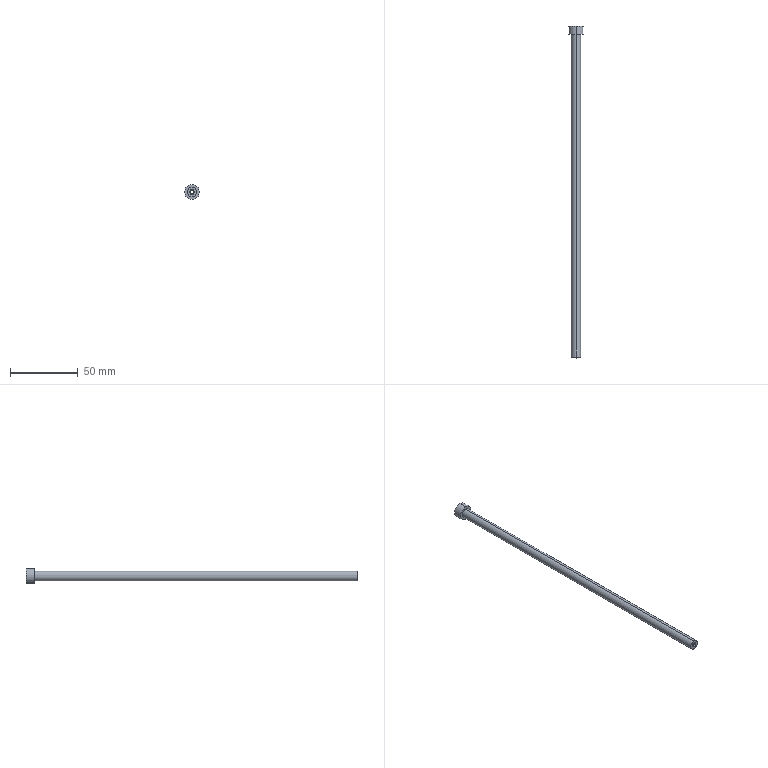Part | STEP file | 1 solid | 13 faces | box 11 x 244.986 x 11 mm | volume 8542 mm3 | cylinder 6 | cone 4 | plane 3 | commonest cylinder face diameters 2.5 x2 7 x2 11 x2
STEP:
#1=CARTESIAN_POINT('',(0.,0.,0.));
#2=DIRECTION('',(0.,0.,1.));
#3=DIRECTION('',(1.,0.,0.));
#4=AXIS2_PLACEMENT_3D('',#1,#2,#3);
#5=CARTESIAN_POINT('',(-37.688,290.5,7.565));
#6=VERTEX_POINT('',#5);
#7=CARTESIAN_POINT('',(-37.688,290.5,18.565));
#8=VERTEX_POINT('',#7);
#9=CARTESIAN_POINT('',(-37.688,290.5,13.065));
#10=DIRECTION('',(0.,-1.,0.));
#11=DIRECTION('',(0.,0.,-1.));
#12=AXIS2_PLACEMENT_3D('',#9,#10,#11);
#13=CIRCLE('',#12,5.5);
#14=CARTESIAN_POINT('',(-37.688,290.5,13.065));
#15=DIRECTION('',(0.,-1.,0.));
#16=DIRECTION('',(0.,0.,-1.));
#17=AXIS2_PLACEMENT_3D('',#14,#15,#16);
#18=CYLINDRICAL_SURFACE('',#17,5.5);
#19=CARTESIAN_POINT('',(0.,0.));
#20=DIRECTION('',(1.,0.));
#21=VECTOR('',#20,1.);
#22=LINE('',#19,#21);
#23=(GEOMETRIC_REPRESENTATION_CONTEXT(2)PARAMETRIC_REPRESENTATION_CONTEXT()REPRESENTATION_CONTEXT('',''));
#24=DEFINITIONAL_REPRESENTATION('',(#22),#23);
#25=PCURVE('',#18,#24);
#26=CARTESIAN_POINT('',(-72.862,290.5,110.196));
#27=DIRECTION('',(0.,-1.,0.));
#28=DIRECTION('',(0.,0.,-1.));
#29=AXIS2_PLACEMENT_3D('',#26,#27,#28);
#30=PLANE('',#29);
#31=CARTESIAN_POINT('',(97.131,35.175));
#32=DIRECTION('',(1.,0.));
#33=AXIS2_PLACEMENT_2D('',#31,#32);
#34=CIRCLE('',#33,5.5);
#35=(GEOMETRIC_REPRESENTATION_CONTEXT(2)PARAMETRIC_REPRESENTATION_CONTEXT()REPRESENTATION_CONTEXT('',''));
#36=DEFINITIONAL_REPRESENTATION('',(#34),#35);
#37=PCURVE('',#30,#36);
#38=SURFACE_CURVE('',#13,(#25,#37),.PCURVE_S1.);
#39=EDGE_CURVE('',#6,#8,#38,.T.);
#40=ORIENTED_EDGE('',*,*,#39,.T.);
#41=CARTESIAN_POINT('',(-37.688,284.5,18.565));
#42=VERTEX_POINT('',#41);
#43=CARTESIAN_POINT('',(-37.688,290.5,18.565));
#44=DIRECTION('',(0.,-1.,0.));
#45=VECTOR('',#44,1.);
#46=LINE('',#43,#45);
#47=CARTESIAN_POINT('',(3.142,0.));
#48=DIRECTION('',(0.,1.));
#49=VECTOR('',#48,1.);
#50=LINE('',#47,#49);
#51=(GEOMETRIC_REPRESENTATION_CONTEXT(2)PARAMETRIC_REPRESENTATION_CONTEXT()REPRESENTATION_CONTEXT('',''));
#52=DEFINITIONAL_REPRESENTATION('',(#50),#51);
#53=PCURVE('',#18,#52);
#54=CARTESIAN_POINT('',(-37.688,290.5,13.065));
#55=DIRECTION('',(0.,-1.,0.));
#56=DIRECTION('',(0.,0.,-1.));
#57=AXIS2_PLACEMENT_3D('',#54,#55,#56);
#58=CYLINDRICAL_SURFACE('',#57,5.5);
#59=CARTESIAN_POINT('',(3.142,0.));
#60=DIRECTION('',(0.,1.));
#61=VECTOR('',#60,1.);
#62=LINE('',#59,#61);
#63=(GEOMETRIC_REPRESENTATION_CONTEXT(2)PARAMETRIC_REPRESENTATION_CONTEXT()REPRESENTATION_CONTEXT('',''));
#64=DEFINITIONAL_REPRESENTATION('',(#62),#63);
#65=PCURVE('',#58,#64);
#66=SURFACE_CURVE('',#46,(#53,#65),.PCURVE_S1.);
#67=EDGE_CURVE('',#8,#42,#66,.T.);
#68=ORIENTED_EDGE('',*,*,#67,.T.);
#69=CARTESIAN_POINT('',(-37.688,284.5,7.565));
#70=VERTEX_POINT('',#69);
#71=CARTESIAN_POINT('',(-37.688,284.5,13.065));
#72=DIRECTION('',(0.,1.,0.));
#73=DIRECTION('',(0.,0.,1.));
#74=AXIS2_PLACEMENT_3D('',#71,#72,#73);
#75=CIRCLE('',#74,5.5);
#76=CARTESIAN_POINT('',(3.142,6.));
#77=DIRECTION('',(-1.,0.));
#78=VECTOR('',#77,1.);
#79=LINE('',#76,#78);
#80=(GEOMETRIC_REPRESENTATION_CONTEXT(2)PARAMETRIC_REPRESENTATION_CONTEXT()REPRESENTATION_CONTEXT('',''));
#81=DEFINITIONAL_REPRESENTATION('',(#79),#80);
#82=PCURVE('',#18,#81);
#83=CARTESIAN_POINT('',(-37.688,284.5,13.065));
#84=DIRECTION('',(0.,-1.,0.));
#85=DIRECTION('',(0.,0.,-1.));
#86=AXIS2_PLACEMENT_3D('',#83,#84,#85);
#87=PLANE('',#86);
#88=CARTESIAN_POINT('',(-5.5,0.));
#89=CARTESIAN_POINT('',(-5.5,9.526));
#90=CARTESIAN_POINT('',(2.75,4.763));
#91=CARTESIAN_POINT('',(11.,0.));
#92=CARTESIAN_POINT('',(2.75,-4.763));
#93=CARTESIAN_POINT('',(-5.5,-9.526));
#94=CARTESIAN_POINT('',(-5.5,0.));
#95=(BOUNDED_CURVE()B_SPLINE_CURVE(2,(#88,#89,#90,#91,#92,#93,#94),.UNSPECIFIED.,.T.,.F.)B_SPLINE_CURVE_WITH_KNOTS((1,2,2,2,2,1),(-2.094,0.,2.094,4.189,6.283,8.378),.UNSPECIFIED.)CURVE()GEOMETRIC_REPRESENTATION_ITEM()RATIONAL_B_SPLINE_CURVE((1.,0.5,1.,0.5,1.,0.5,1.))REPRESENTATION_ITEM(''));
#96=(GEOMETRIC_REPRESENTATION_CONTEXT(2)PARAMETRIC_REPRESENTATION_CONTEXT()REPRESENTATION_CONTEXT('',''));
#97=DEFINITIONAL_REPRESENTATION('',(#95),#96);
#98=PCURVE('',#87,#97);
#99=SURFACE_CURVE('',#75,(#82,#98),.PCURVE_S1.);
#100=EDGE_CURVE('',#42,#70,#99,.T.);
#101=ORIENTED_EDGE('',*,*,#100,.T.);
#102=CARTESIAN_POINT('',(-37.688,290.5,7.565));
#103=DIRECTION('',(0.,-1.,0.));
#104=VECTOR('',#103,1.);
#105=LINE('',#102,#104);
#106=CARTESIAN_POINT('',(0.,0.));
#107=DIRECTION('',(0.,1.));
#108=VECTOR('',#107,1.);
#109=LINE('',#106,#108);
#110=(GEOMETRIC_REPRESENTATION_CONTEXT(2)PARAMETRIC_REPRESENTATION_CONTEXT()REPRESENTATION_CONTEXT('',''));
#111=DEFINITIONAL_REPRESENTATION('',(#109),#110);
#112=PCURVE('',#18,#111);
#113=CARTESIAN_POINT('',(6.283,0.));
#114=DIRECTION('',(0.,1.));
#115=VECTOR('',#114,1.);
#116=LINE('',#113,#115);
#117=(GEOMETRIC_REPRESENTATION_CONTEXT(2)PARAMETRIC_REPRESENTATION_CONTEXT()REPRESENTATION_CONTEXT('',''));
#118=DEFINITIONAL_REPRESENTATION('',(#116),#117);
#119=PCURVE('',#58,#118);
#120=SURFACE_CURVE('',#105,(#112,#119),.PCURVE_S1.);
#121=EDGE_CURVE('',#6,#70,#120,.T.);
#122=ORIENTED_EDGE('',*,*,#121,.F.);
#123=EDGE_LOOP('',(#40,#68,#101,#122));
#124=FACE_BOUND('',#123,.T.);
#125=ADVANCED_FACE('',(#124),#18,.T.);
#126=CARTESIAN_POINT('',(-37.688,45.514,14.315));
#127=VERTEX_POINT('',#126);
#128=CARTESIAN_POINT('',(-37.688,290.5,14.315));
#129=VERTEX_POINT('',#128);
#130=CARTESIAN_POINT('',(-37.688,33.165,14.315));
#131=DIRECTION('',(0.,1.,0.));
#132=VECTOR('',#131,1.);
#133=LINE('',#130,#132);
#134=CARTESIAN_POINT('',(-37.688,33.165,13.065));
#135=DIRECTION('',(0.,1.,0.));
#136=DIRECTION('',(0.,0.,1.));
#137=AXIS2_PLACEMENT_3D('',#134,#135,#136);
#138=CYLINDRICAL_SURFACE('',#137,1.25);
#139=CARTESIAN_POINT('',(6.283,0.));
#140=DIRECTION('',(0.,1.));
#141=VECTOR('',#140,1.);
#142=LINE('',#139,#141);
#143=(GEOMETRIC_REPRESENTATION_CONTEXT(2)PARAMETRIC_REPRESENTATION_CONTEXT()REPRESENTATION_CONTEXT('',''));
#144=DEFINITIONAL_REPRESENTATION('',(#142),#143);
#145=PCURVE('',#138,#144);
#146=CARTESIAN_POINT('',(-37.688,33.165,13.065));
#147=DIRECTION('',(0.,1.,0.));
#148=DIRECTION('',(0.,0.,1.));
#149=AXIS2_PLACEMENT_3D('',#146,#147,#148);
#150=CYLINDRICAL_SURFACE('',#149,1.25);
#151=CARTESIAN_POINT('',(0.,0.));
#152=DIRECTION('',(0.,1.));
#153=VECTOR('',#152,1.);
#154=LINE('',#151,#153);
#155=(GEOMETRIC_REPRESENTATION_CONTEXT(2)PARAMETRIC_REPRESENTATION_CONTEXT()REPRESENTATION_CONTEXT('',''));
#156=DEFINITIONAL_REPRESENTATION('',(#154),#155);
#157=PCURVE('',#150,#156);
#158=SURFACE_CURVE('',#133,(#145,#157),.PCURVE_S1.);
#159=EDGE_CURVE('',#127,#129,#158,.T.);
#160=ORIENTED_EDGE('',*,*,#159,.T.);
#161=CARTESIAN_POINT('',(-37.688,290.5,11.815));
#162=VERTEX_POINT('',#161);
#163=CARTESIAN_POINT('',(-37.688,290.5,13.065));
#164=DIRECTION('',(0.,-1.,0.));
#165=DIRECTION('',(0.,0.,-1.));
#166=AXIS2_PLACEMENT_3D('',#163,#164,#165);
#167=CIRCLE('',#166,1.25);
#168=CARTESIAN_POINT('',(9.425,257.335));
#169=DIRECTION('',(-1.,0.));
#170=VECTOR('',#169,1.);
#171=LINE('',#168,#170);
#172=(GEOMETRIC_REPRESENTATION_CONTEXT(2)PARAMETRIC_REPRESENTATION_CONTEXT()REPRESENTATION_CONTEXT('',''));
#173=DEFINITIONAL_REPRESENTATION('',(#171),#172);
#174=PCURVE('',#138,#173);
#175=CARTESIAN_POINT('',(97.131,35.175));
#176=DIRECTION('',(1.,0.));
#177=AXIS2_PLACEMENT_2D('',#175,#176);
#178=CIRCLE('',#177,1.25);
#179=(GEOMETRIC_REPRESENTATION_CONTEXT(2)PARAMETRIC_REPRESENTATION_CONTEXT()REPRESENTATION_CONTEXT('',''));
#180=DEFINITIONAL_REPRESENTATION('',(#178),#179);
#181=PCURVE('',#30,#180);
#182=SURFACE_CURVE('',#167,(#174,#181),.PCURVE_S1.);
#183=EDGE_CURVE('',#129,#162,#182,.T.);
#184=ORIENTED_EDGE('',*,*,#183,.T.);
#185=CARTESIAN_POINT('',(-37.688,45.514,11.815));
#186=VERTEX_POINT('',#185);
#187=CARTESIAN_POINT('',(-37.688,33.165,11.815));
#188=DIRECTION('',(0.,1.,0.));
#189=VECTOR('',#188,1.);
#190=LINE('',#187,#189);
#191=CARTESIAN_POINT('',(3.142,0.));
#192=DIRECTION('',(0.,1.));
#193=VECTOR('',#192,1.);
#194=LINE('',#191,#193);
#195=(GEOMETRIC_REPRESENTATION_CONTEXT(2)PARAMETRIC_REPRESENTATION_CONTEXT()REPRESENTATION_CONTEXT('',''));
#196=DEFINITIONAL_REPRESENTATION('',(#194),#195);
#197=PCURVE('',#138,#196);
#198=CARTESIAN_POINT('',(3.142,0.));
#199=DIRECTION('',(0.,1.));
#200=VECTOR('',#199,1.);
#201=LINE('',#198,#200);
#202=(GEOMETRIC_REPRESENTATION_CONTEXT(2)PARAMETRIC_REPRESENTATION_CONTEXT()REPRESENTATION_CONTEXT('',''));
#203=DEFINITIONAL_REPRESENTATION('',(#201),#202);
#204=PCURVE('',#150,#203);
#205=SURFACE_CURVE('',#190,(#197,#204),.PCURVE_S1.);
#206=EDGE_CURVE('',#186,#162,#205,.T.);
#207=ORIENTED_EDGE('',*,*,#206,.F.);
#208=CARTESIAN_POINT('',(-37.688,45.514,13.065));
#209=DIRECTION('',(0.,1.,0.));
#210=DIRECTION('',(0.,0.,1.));
#211=AXIS2_PLACEMENT_3D('',#208,#209,#210);
#212=CIRCLE('',#211,1.25);
#213=CARTESIAN_POINT('',(0.,12.349));
#214=DIRECTION('',(1.,0.));
#215=VECTOR('',#214,1.);
#216=LINE('',#213,#215);
#217=(GEOMETRIC_REPRESENTATION_CONTEXT(2)PARAMETRIC_REPRESENTATION_CONTEXT()REPRESENTATION_CONTEXT('',''));
#218=DEFINITIONAL_REPRESENTATION('',(#216),#217);
#219=PCURVE('',#138,#218);
#220=CARTESIAN_POINT('',(-37.688,46.23,13.065));
#221=DIRECTION('',(0.,1.,0.));
#222=DIRECTION('',(0.,0.,1.));
#223=AXIS2_PLACEMENT_3D('',#220,#221,#222);
#224=CONICAL_SURFACE('',#223,1.256,0.008727);
#225=CARTESIAN_POINT('',(0.,-0.7162));
#226=DIRECTION('',(1.,0.));
#227=VECTOR('',#226,1.);
#228=LINE('',#225,#227);
#229=(GEOMETRIC_REPRESENTATION_CONTEXT(2)PARAMETRIC_REPRESENTATION_CONTEXT()REPRESENTATION_CONTEXT('',''));
#230=DEFINITIONAL_REPRESENTATION('',(#228),#229);
#231=PCURVE('',#224,#230);
#232=SURFACE_CURVE('',#212,(#219,#231),.PCURVE_S1.);
#233=EDGE_CURVE('',#186,#127,#232,.T.);
#234=ORIENTED_EDGE('',*,*,#233,.T.);
#235=EDGE_LOOP('',(#160,#184,#207,#234));
#236=FACE_BOUND('',#235,.F.);
#237=ADVANCED_FACE('',(#236),#138,.F.);
#238=CARTESIAN_POINT('',(-37.688,46.23,9.565));
#239=VERTEX_POINT('',#238);
#240=CARTESIAN_POINT('',(-37.688,46.23,16.565));
#241=VERTEX_POINT('',#240);
#242=CARTESIAN_POINT('',(-37.688,46.23,13.065));
#243=DIRECTION('',(0.,-1.,0.));
#244=DIRECTION('',(0.,0.,1.));
#245=AXIS2_PLACEMENT_3D('',#242,#243,#244);
#246=CIRCLE('',#245,3.5);
#247=CARTESIAN_POINT('',(-37.688,33.165,13.065));
#248=DIRECTION('',(0.,1.,0.));
#249=DIRECTION('',(0.,0.,1.));
#250=AXIS2_PLACEMENT_3D('',#247,#248,#249);
#251=CYLINDRICAL_SURFACE('',#250,3.5);
#252=CARTESIAN_POINT('',(6.283,13.065));
#253=DIRECTION('',(-1.,0.));
#254=VECTOR('',#253,1.);
#255=LINE('',#252,#254);
#256=(GEOMETRIC_REPRESENTATION_CONTEXT(2)PARAMETRIC_REPRESENTATION_CONTEXT()REPRESENTATION_CONTEXT('',''));
#257=DEFINITIONAL_REPRESENTATION('',(#255),#256);
#258=PCURVE('',#251,#257);
#259=CARTESIAN_POINT('',(-37.688,46.23,13.065));
#260=DIRECTION('',(0.,1.,0.));
#261=DIRECTION('',(0.,0.,1.));
#262=AXIS2_PLACEMENT_3D('',#259,#260,#261);
#263=PLANE('',#262);
#264=CARTESIAN_POINT('',(3.5,0.));
#265=CARTESIAN_POINT('',(3.5,-6.062));
#266=CARTESIAN_POINT('',(-1.75,-3.031));
#267=CARTESIAN_POINT('',(-7.,0.));
#268=CARTESIAN_POINT('',(-1.75,3.031));
#269=CARTESIAN_POINT('',(3.5,6.062));
#270=CARTESIAN_POINT('',(3.5,0.));
#271=(BOUNDED_CURVE()B_SPLINE_CURVE(2,(#264,#265,#266,#267,#268,#269,#270),.UNSPECIFIED.,.T.,.F.)B_SPLINE_CURVE_WITH_KNOTS((1,2,2,2,2,1),(-2.094,0.,2.094,4.189,6.283,8.378),.UNSPECIFIED.)CURVE()GEOMETRIC_REPRESENTATION_ITEM()RATIONAL_B_SPLINE_CURVE((1.,0.5,1.,0.5,1.,0.5,1.))REPRESENTATION_ITEM(''));
#272=(GEOMETRIC_REPRESENTATION_CONTEXT(2)PARAMETRIC_REPRESENTATION_CONTEXT()REPRESENTATION_CONTEXT('',''));
#273=DEFINITIONAL_REPRESENTATION('',(#271),#272);
#274=PCURVE('',#263,#273);
#275=SURFACE_CURVE('',#246,(#258,#274),.PCURVE_S1.);
#276=EDGE_CURVE('',#239,#241,#275,.T.);
#277=ORIENTED_EDGE('',*,*,#276,.F.);
#278=CARTESIAN_POINT('',(-37.688,284.5,9.565));
#279=VERTEX_POINT('',#278);
#280=CARTESIAN_POINT('',(-37.688,33.165,9.565));
#281=DIRECTION('',(0.,1.,0.));
#282=VECTOR('',#281,1.);
#283=LINE('',#280,#282);
#284=CARTESIAN_POINT('',(3.142,0.));
#285=DIRECTION('',(0.,1.));
#286=VECTOR('',#285,1.);
#287=LINE('',#284,#286);
#288=(GEOMETRIC_REPRESENTATION_CONTEXT(2)PARAMETRIC_REPRESENTATION_CONTEXT()REPRESENTATION_CONTEXT('',''));
#289=DEFINITIONAL_REPRESENTATION('',(#287),#288);
#290=PCURVE('',#251,#289);
#291=CARTESIAN_POINT('',(-37.688,33.165,13.065));
#292=DIRECTION('',(0.,1.,0.));
#293=DIRECTION('',(0.,0.,1.));
#294=AXIS2_PLACEMENT_3D('',#291,#292,#293);
#295=CYLINDRICAL_SURFACE('',#294,3.5);
#296=CARTESIAN_POINT('',(3.142,0.));
#297=DIRECTION('',(0.,1.));
#298=VECTOR('',#297,1.);
#299=LINE('',#296,#298);
#300=(GEOMETRIC_REPRESENTATION_CONTEXT(2)PARAMETRIC_REPRESENTATION_CONTEXT()REPRESENTATION_CONTEXT('',''));
#301=DEFINITIONAL_REPRESENTATION('',(#299),#300);
#302=PCURVE('',#295,#301);
#303=SURFACE_CURVE('',#283,(#290,#302),.PCURVE_S1.);
#304=EDGE_CURVE('',#239,#279,#303,.T.);
#305=ORIENTED_EDGE('',*,*,#304,.T.);
#306=CARTESIAN_POINT('',(-37.688,284.5,16.565));
#307=VERTEX_POINT('',#306);
#308=CARTESIAN_POINT('',(-37.688,284.5,13.065));
#309=DIRECTION('',(0.,1.,0.));
#310=DIRECTION('',(0.,0.,-1.));
#311=AXIS2_PLACEMENT_3D('',#308,#309,#310);
#312=CIRCLE('',#311,3.5);
#313=CARTESIAN_POINT('',(-3.142,251.335));
#314=DIRECTION('',(1.,0.));
#315=VECTOR('',#314,1.);
#316=LINE('',#313,#315);
#317=(GEOMETRIC_REPRESENTATION_CONTEXT(2)PARAMETRIC_REPRESENTATION_CONTEXT()REPRESENTATION_CONTEXT('',''));
#318=DEFINITIONAL_REPRESENTATION('',(#316),#317);
#319=PCURVE('',#251,#318);
#320=CARTESIAN_POINT('',(3.5,0.));
#321=CARTESIAN_POINT('',(3.5,-6.062));
#322=CARTESIAN_POINT('',(-1.75,-3.031));
#323=CARTESIAN_POINT('',(-7.,0.));
#324=CARTESIAN_POINT('',(-1.75,3.031));
#325=CARTESIAN_POINT('',(3.5,6.062));
#326=CARTESIAN_POINT('',(3.5,0.));
#327=(BOUNDED_CURVE()B_SPLINE_CURVE(2,(#320,#321,#322,#323,#324,#325,#326),.UNSPECIFIED.,.T.,.F.)B_SPLINE_CURVE_WITH_KNOTS((1,2,2,2,2,1),(-2.094,0.,2.094,4.189,6.283,8.378),.UNSPECIFIED.)CURVE()GEOMETRIC_REPRESENTATION_ITEM()RATIONAL_B_SPLINE_CURVE((1.,0.5,1.,0.5,1.,0.5,1.))REPRESENTATION_ITEM(''));
#328=(GEOMETRIC_REPRESENTATION_CONTEXT(2)PARAMETRIC_REPRESENTATION_CONTEXT()REPRESENTATION_CONTEXT('',''));
#329=DEFINITIONAL_REPRESENTATION('',(#327),#328);
#330=PCURVE('',#87,#329);
#331=SURFACE_CURVE('',#312,(#319,#330),.PCURVE_S1.);
#332=EDGE_CURVE('',#307,#279,#331,.T.);
#333=ORIENTED_EDGE('',*,*,#332,.F.);
#334=CARTESIAN_POINT('',(-37.688,33.165,16.565));
#335=DIRECTION('',(0.,1.,0.));
#336=VECTOR('',#335,1.);
#337=LINE('',#334,#336);
#338=CARTESIAN_POINT('',(0.,0.));
#339=DIRECTION('',(0.,1.));
#340=VECTOR('',#339,1.);
#341=LINE('',#338,#340);
#342=(GEOMETRIC_REPRESENTATION_CONTEXT(2)PARAMETRIC_REPRESENTATION_CONTEXT()REPRESENTATION_CONTEXT('',''));
#343=DEFINITIONAL_REPRESENTATION('',(#341),#342);
#344=PCURVE('',#251,#343);
#345=CARTESIAN_POINT('',(6.283,0.));
#346=DIRECTION('',(0.,1.));
#347=VECTOR('',#346,1.);
#348=LINE('',#345,#347);
#349=(GEOMETRIC_REPRESENTATION_CONTEXT(2)PARAMETRIC_REPRESENTATION_CONTEXT()REPRESENTATION_CONTEXT('',''));
#350=DEFINITIONAL_REPRESENTATION('',(#348),#349);
#351=PCURVE('',#295,#350);
#352=SURFACE_CURVE('',#337,(#344,#351),.PCURVE_S1.);
#353=EDGE_CURVE('',#241,#307,#352,.T.);
#354=ORIENTED_EDGE('',*,*,#353,.F.);
#355=EDGE_LOOP('',(#277,#305,#333,#354));
#356=FACE_BOUND('',#355,.T.);
#357=ADVANCED_FACE('',(#356),#251,.T.);
#358=CARTESIAN_POINT('',(-37.688,45.723,14.317));
#359=VERTEX_POINT('',#358);
#360=CARTESIAN_POINT('',(-37.688,45.723,11.813));
#361=VERTEX_POINT('',#360);
#362=CARTESIAN_POINT('',(-37.688,45.723,13.065));
#363=DIRECTION('',(0.,1.,0.));
#364=DIRECTION('',(0.,0.,1.));
#365=AXIS2_PLACEMENT_3D('',#362,#363,#364);
#366=CIRCLE('',#365,1.252);
#367=CARTESIAN_POINT('',(-37.688,45.723,13.065));
#368=DIRECTION('',(0.,1.,0.));
#369=DIRECTION('',(0.,0.,1.));
#370=AXIS2_PLACEMENT_3D('',#367,#368,#369);
#371=CONICAL_SURFACE('',#370,1.252,0.7854);
#372=CARTESIAN_POINT('',(0.,0.));
#373=DIRECTION('',(1.,0.));
#374=VECTOR('',#373,1.);
#375=LINE('',#372,#374);
#376=(GEOMETRIC_REPRESENTATION_CONTEXT(2)PARAMETRIC_REPRESENTATION_CONTEXT()REPRESENTATION_CONTEXT('',''));
#377=DEFINITIONAL_REPRESENTATION('',(#375),#376);
#378=PCURVE('',#371,#377);
#379=CARTESIAN_POINT('',(-37.688,46.23,13.065));
#380=DIRECTION('',(0.,1.,0.));
#381=DIRECTION('',(0.,0.,1.));
#382=AXIS2_PLACEMENT_3D('',#379,#380,#381);
#383=CONICAL_SURFACE('',#382,1.256,0.008727);
#384=CARTESIAN_POINT('',(0.,-0.5069));
#385=DIRECTION('',(1.,0.));
#386=VECTOR('',#385,1.);
#387=LINE('',#384,#386);
#388=(GEOMETRIC_REPRESENTATION_CONTEXT(2)PARAMETRIC_REPRESENTATION_CONTEXT()REPRESENTATION_CONTEXT('',''));
#389=DEFINITIONAL_REPRESENTATION('',(#387),#388);
#390=PCURVE('',#383,#389);
#391=SURFACE_CURVE('',#366,(#378,#390),.PCURVE_S1.);
#392=EDGE_CURVE('',#359,#361,#391,.T.);
#393=ORIENTED_EDGE('',*,*,#392,.T.);
#394=CARTESIAN_POINT('',(-37.688,46.23,11.306));
#395=VERTEX_POINT('',#394);
#396=CARTESIAN_POINT('',(-37.688,45.723,11.813));
#397=DIRECTION('',(0.,0.7071,-0.7071));
#398=VECTOR('',#397,1.);
#399=LINE('',#396,#398);
#400=CARTESIAN_POINT('',(3.142,0.));
#401=DIRECTION('',(0.,1.));
#402=VECTOR('',#401,1.);
#403=LINE('',#400,#402);
#404=(GEOMETRIC_REPRESENTATION_CONTEXT(2)PARAMETRIC_REPRESENTATION_CONTEXT()REPRESENTATION_CONTEXT('',''));
#405=DEFINITIONAL_REPRESENTATION('',(#403),#404);
#406=PCURVE('',#371,#405);
#407=CARTESIAN_POINT('',(-37.688,45.723,13.065));
#408=DIRECTION('',(0.,1.,0.));
#409=DIRECTION('',(0.,0.,1.));
#410=AXIS2_PLACEMENT_3D('',#407,#408,#409);
#411=CONICAL_SURFACE('',#410,1.252,0.7854);
#412=CARTESIAN_POINT('',(3.142,0.));
#413=DIRECTION('',(0.,1.));
#414=VECTOR('',#413,1.);
#415=LINE('',#412,#414);
#416=(GEOMETRIC_REPRESENTATION_CONTEXT(2)PARAMETRIC_REPRESENTATION_CONTEXT()REPRESENTATION_CONTEXT('',''));
#417=DEFINITIONAL_REPRESENTATION('',(#415),#416);
#418=PCURVE('',#411,#417);
#419=SURFACE_CURVE('',#399,(#406,#418),.PCURVE_S1.);
#420=EDGE_CURVE('',#361,#395,#419,.T.);
#421=ORIENTED_EDGE('',*,*,#420,.T.);
#422=CARTESIAN_POINT('',(-37.688,46.23,14.824));
#423=VERTEX_POINT('',#422);
#424=CARTESIAN_POINT('',(-37.688,46.23,13.065));
#425=DIRECTION('',(0.,-1.,0.));
#426=DIRECTION('',(0.,0.,1.));
#427=AXIS2_PLACEMENT_3D('',#424,#425,#426);
#428=CIRCLE('',#427,1.759);
#429=CARTESIAN_POINT('',(6.283,0.5069));
#430=DIRECTION('',(-1.,0.));
#431=VECTOR('',#430,1.);
#432=LINE('',#429,#431);
#433=(GEOMETRIC_REPRESENTATION_CONTEXT(2)PARAMETRIC_REPRESENTATION_CONTEXT()REPRESENTATION_CONTEXT('',''));
#434=DEFINITIONAL_REPRESENTATION('',(#432),#433);
#435=PCURVE('',#371,#434);
#436=CARTESIAN_POINT('',(1.759,0.));
#437=CARTESIAN_POINT('',(1.759,-3.046));
#438=CARTESIAN_POINT('',(-0.8794,-1.523));
#439=CARTESIAN_POINT('',(-3.518,0.));
#440=CARTESIAN_POINT('',(-0.8794,1.523));
#441=CARTESIAN_POINT('',(1.759,3.046));
#442=CARTESIAN_POINT('',(1.759,0.));
#443=(BOUNDED_CURVE()B_SPLINE_CURVE(2,(#436,#437,#438,#439,#440,#441,#442),.UNSPECIFIED.,.T.,.F.)B_SPLINE_CURVE_WITH_KNOTS((1,2,2,2,2,1),(-2.094,0.,2.094,4.189,6.283,8.378),.UNSPECIFIED.)CURVE()GEOMETRIC_REPRESENTATION_ITEM()RATIONAL_B_SPLINE_CURVE((1.,0.5,1.,0.5,1.,0.5,1.))REPRESENTATION_ITEM(''));
#444=(GEOMETRIC_REPRESENTATION_CONTEXT(2)PARAMETRIC_REPRESENTATION_CONTEXT()REPRESENTATION_CONTEXT('',''));
#445=DEFINITIONAL_REPRESENTATION('',(#443),#444);
#446=PCURVE('',#263,#445);
#447=SURFACE_CURVE('',#428,(#435,#446),.PCURVE_S1.);
#448=EDGE_CURVE('',#395,#423,#447,.T.);
#449=ORIENTED_EDGE('',*,*,#448,.T.);
#450=CARTESIAN_POINT('',(-37.688,45.723,14.317));
#451=DIRECTION('',(0.,0.7071,0.7071));
#452=VECTOR('',#451,1.);
#453=LINE('',#450,#452);
#454=CARTESIAN_POINT('',(0.,0.));
#455=DIRECTION('',(0.,1.));
#456=VECTOR('',#455,1.);
#457=LINE('',#454,#456);
#458=(GEOMETRIC_REPRESENTATION_CONTEXT(2)PARAMETRIC_REPRESENTATION_CONTEXT()REPRESENTATION_CONTEXT('',''));
#459=DEFINITIONAL_REPRESENTATION('',(#457),#458);
#460=PCURVE('',#371,#459);
#461=CARTESIAN_POINT('',(6.283,0.));
#462=DIRECTION('',(0.,1.));
#463=VECTOR('',#462,1.);
#464=LINE('',#461,#463);
#465=(GEOMETRIC_REPRESENTATION_CONTEXT(2)PARAMETRIC_REPRESENTATION_CONTEXT()REPRESENTATION_CONTEXT('',''));
#466=DEFINITIONAL_REPRESENTATION('',(#464),#465);
#467=PCURVE('',#411,#466);
#468=SURFACE_CURVE('',#453,(#460,#467),.PCURVE_S1.);
#469=EDGE_CURVE('',#359,#423,#468,.T.);
#470=ORIENTED_EDGE('',*,*,#469,.F.);
#471=EDGE_LOOP('',(#393,#421,#449,#470));
#472=FACE_BOUND('',#471,.T.);
#473=ADVANCED_FACE('',(#472),#371,.T.);
#474=CARTESIAN_POINT('',(-37.688,45.514,13.065));
#475=DIRECTION('',(0.,1.,0.));
#476=DIRECTION('',(0.,0.,1.));
#477=AXIS2_PLACEMENT_3D('',#474,#475,#476);
#478=CIRCLE('',#477,1.25);
#479=CARTESIAN_POINT('',(0.,-0.7162));
#480=DIRECTION('',(1.,0.));
#481=VECTOR('',#480,1.);
#482=LINE('',#479,#481);
#483=(GEOMETRIC_REPRESENTATION_CONTEXT(2)PARAMETRIC_REPRESENTATION_CONTEXT()REPRESENTATION_CONTEXT('',''));
#484=DEFINITIONAL_REPRESENTATION('',(#482),#483);
#485=PCURVE('',#383,#484);
#486=CARTESIAN_POINT('',(0.,12.349));
#487=DIRECTION('',(1.,0.));
#488=VECTOR('',#487,1.);
#489=LINE('',#486,#488);
#490=(GEOMETRIC_REPRESENTATION_CONTEXT(2)PARAMETRIC_REPRESENTATION_CONTEXT()REPRESENTATION_CONTEXT('',''));
#491=DEFINITIONAL_REPRESENTATION('',(#489),#490);
#492=PCURVE('',#150,#491);
#493=SURFACE_CURVE('',#478,(#485,#492),.PCURVE_S1.);
#494=EDGE_CURVE('',#127,#186,#493,.T.);
#495=ORIENTED_EDGE('',*,*,#494,.T.);
#496=CARTESIAN_POINT('',(-37.688,46.23,11.809));
#497=DIRECTION('',(0.,1.,-0.008727));
#498=VECTOR('',#497,1.);
#499=LINE('',#496,#498);
#500=CARTESIAN_POINT('',(3.142,0.));
#501=DIRECTION('',(0.,1.));
#502=VECTOR('',#501,1.);
#503=LINE('',#500,#502);
#504=(GEOMETRIC_REPRESENTATION_CONTEXT(2)PARAMETRIC_REPRESENTATION_CONTEXT()REPRESENTATION_CONTEXT('',''));
#505=DEFINITIONAL_REPRESENTATION('',(#503),#504);
#506=PCURVE('',#383,#505);
#507=CARTESIAN_POINT('',(3.142,0.));
#508=DIRECTION('',(0.,1.));
#509=VECTOR('',#508,1.);
#510=LINE('',#507,#509);
#511=(GEOMETRIC_REPRESENTATION_CONTEXT(2)PARAMETRIC_REPRESENTATION_CONTEXT()REPRESENTATION_CONTEXT('',''));
#512=DEFINITIONAL_REPRESENTATION('',(#510),#511);
#513=PCURVE('',#224,#512);
#514=SURFACE_CURVE('',#499,(#506,#513),.PCURVE_S1.);
#515=EDGE_CURVE('',#186,#361,#514,.T.);
#516=ORIENTED_EDGE('',*,*,#515,.T.);
#517=ORIENTED_EDGE('',*,*,#392,.F.);
#518=CARTESIAN_POINT('',(-37.688,46.23,14.321));
#519=DIRECTION('',(0.,1.,0.008727));
#520=VECTOR('',#519,1.);
#521=LINE('',#518,#520);
#522=CARTESIAN_POINT('',(0.,0.));
#523=DIRECTION('',(0.,1.));
#524=VECTOR('',#523,1.);
#525=LINE('',#522,#524);
#526=(GEOMETRIC_REPRESENTATION_CONTEXT(2)PARAMETRIC_REPRESENTATION_CONTEXT()REPRESENTATION_CONTEXT('',''));
#527=DEFINITIONAL_REPRESENTATION('',(#525),#526);
#528=PCURVE('',#383,#527);
#529=CARTESIAN_POINT('',(6.283,0.));
#530=DIRECTION('',(0.,1.));
#531=VECTOR('',#530,1.);
#532=LINE('',#529,#531);
#533=(GEOMETRIC_REPRESENTATION_CONTEXT(2)PARAMETRIC_REPRESENTATION_CONTEXT()REPRESENTATION_CONTEXT('',''));
#534=DEFINITIONAL_REPRESENTATION('',(#532),#533);
#535=PCURVE('',#224,#534);
#536=SURFACE_CURVE('',#521,(#528,#535),.PCURVE_S1.);
#537=EDGE_CURVE('',#127,#359,#536,.T.);
#538=ORIENTED_EDGE('',*,*,#537,.F.);
#539=EDGE_LOOP('',(#495,#516,#517,#538));
#540=FACE_BOUND('',#539,.T.);
#541=ADVANCED_FACE('',(#540),#383,.T.);
#542=ORIENTED_EDGE('',*,*,#515,.F.);
#543=ORIENTED_EDGE('',*,*,#233,.T.);
#544=ORIENTED_EDGE('',*,*,#537,.T.);
#545=CARTESIAN_POINT('',(-37.688,45.723,13.065));
#546=DIRECTION('',(0.,1.,0.));
#547=DIRECTION('',(0.,0.,1.));
#548=AXIS2_PLACEMENT_3D('',#545,#546,#547);
#549=CIRCLE('',#548,1.252);
#550=CARTESIAN_POINT('',(0.,-0.5069));
#551=DIRECTION('',(1.,0.));
#552=VECTOR('',#551,1.);
#553=LINE('',#550,#552);
#554=(GEOMETRIC_REPRESENTATION_CONTEXT(2)PARAMETRIC_REPRESENTATION_CONTEXT()REPRESENTATION_CONTEXT('',''));
#555=DEFINITIONAL_REPRESENTATION('',(#553),#554);
#556=PCURVE('',#224,#555);
#557=CARTESIAN_POINT('',(0.,0.));
#558=DIRECTION('',(1.,0.));
#559=VECTOR('',#558,1.);
#560=LINE('',#557,#559);
#561=(GEOMETRIC_REPRESENTATION_CONTEXT(2)PARAMETRIC_REPRESENTATION_CONTEXT()REPRESENTATION_CONTEXT('',''));
#562=DEFINITIONAL_REPRESENTATION('',(#560),#561);
#563=PCURVE('',#411,#562);
#564=SURFACE_CURVE('',#549,(#556,#563),.PCURVE_S1.);
#565=EDGE_CURVE('',#361,#359,#564,.T.);
#566=ORIENTED_EDGE('',*,*,#565,.F.);
#567=EDGE_LOOP('',(#542,#543,#544,#566));
#568=FACE_BOUND('',#567,.T.);
#569=ADVANCED_FACE('',(#568),#224,.T.);
#570=ORIENTED_EDGE('',*,*,#420,.F.);
#571=ORIENTED_EDGE('',*,*,#565,.T.);
#572=ORIENTED_EDGE('',*,*,#469,.T.);
#573=CARTESIAN_POINT('',(-37.688,46.23,13.065));
#574=DIRECTION('',(0.,-1.,0.));
#575=DIRECTION('',(0.,0.,1.));
#576=AXIS2_PLACEMENT_3D('',#573,#574,#575);
#577=CIRCLE('',#576,1.759);
#578=CARTESIAN_POINT('',(6.283,0.5069));
#579=DIRECTION('',(-1.,0.));
#580=VECTOR('',#579,1.);
#581=LINE('',#578,#580);
#582=(GEOMETRIC_REPRESENTATION_CONTEXT(2)PARAMETRIC_REPRESENTATION_CONTEXT()REPRESENTATION_CONTEXT('',''));
#583=DEFINITIONAL_REPRESENTATION('',(#581),#582);
#584=PCURVE('',#411,#583);
#585=CARTESIAN_POINT('',(1.759,0.));
#586=CARTESIAN_POINT('',(1.759,-3.046));
#587=CARTESIAN_POINT('',(-0.8794,-1.523));
#588=CARTESIAN_POINT('',(-3.518,0.));
#589=CARTESIAN_POINT('',(-0.8794,1.523));
#590=CARTESIAN_POINT('',(1.759,3.046));
#591=CARTESIAN_POINT('',(1.759,0.));
#592=(BOUNDED_CURVE()B_SPLINE_CURVE(2,(#585,#586,#587,#588,#589,#590,#591),.UNSPECIFIED.,.T.,.F.)B_SPLINE_CURVE_WITH_KNOTS((1,2,2,2,2,1),(-2.094,0.,2.094,4.189,6.283,8.378),.UNSPECIFIED.)CURVE()GEOMETRIC_REPRESENTATION_ITEM()RATIONAL_B_SPLINE_CURVE((1.,0.5,1.,0.5,1.,0.5,1.))REPRESENTATION_ITEM(''));
#593=(GEOMETRIC_REPRESENTATION_CONTEXT(2)PARAMETRIC_REPRESENTATION_CONTEXT()REPRESENTATION_CONTEXT('',''));
#594=DEFINITIONAL_REPRESENTATION('',(#592),#593);
#595=PCURVE('',#263,#594);
#596=SURFACE_CURVE('',#577,(#584,#595),.PCURVE_S1.);
#597=EDGE_CURVE('',#423,#395,#596,.T.);
#598=ORIENTED_EDGE('',*,*,#597,.T.);
#599=EDGE_LOOP('',(#570,#571,#572,#598));
#600=FACE_BOUND('',#599,.T.);
#601=ADVANCED_FACE('',(#600),#411,.T.);
#602=CARTESIAN_POINT('',(-37.688,46.23,13.065));
#603=DIRECTION('',(0.,-1.,0.));
#604=DIRECTION('',(0.,0.,1.));
#605=AXIS2_PLACEMENT_3D('',#602,#603,#604);
#606=CIRCLE('',#605,3.5);
#607=CARTESIAN_POINT('',(3.5,0.));
#608=CARTESIAN_POINT('',(3.5,-6.062));
#609=CARTESIAN_POINT('',(-1.75,-3.031));
#610=CARTESIAN_POINT('',(-7.,0.));
#611=CARTESIAN_POINT('',(-1.75,3.031));
#612=CARTESIAN_POINT('',(3.5,6.062));
#613=CARTESIAN_POINT('',(3.5,0.));
#614=(BOUNDED_CURVE()B_SPLINE_CURVE(2,(#607,#608,#609,#610,#611,#612,#613),.UNSPECIFIED.,.T.,.F.)B_SPLINE_CURVE_WITH_KNOTS((1,2,2,2,2,1),(-2.094,0.,2.094,4.189,6.283,8.378),.UNSPECIFIED.)CURVE()GEOMETRIC_REPRESENTATION_ITEM()RATIONAL_B_SPLINE_CURVE((1.,0.5,1.,0.5,1.,0.5,1.))REPRESENTATION_ITEM(''));
#615=(GEOMETRIC_REPRESENTATION_CONTEXT(2)PARAMETRIC_REPRESENTATION_CONTEXT()REPRESENTATION_CONTEXT('',''));
#616=DEFINITIONAL_REPRESENTATION('',(#614),#615);
#617=PCURVE('',#263,#616);
#618=CARTESIAN_POINT('',(6.283,13.065));
#619=DIRECTION('',(-1.,0.));
#620=VECTOR('',#619,1.);
#621=LINE('',#618,#620);
#622=(GEOMETRIC_REPRESENTATION_CONTEXT(2)PARAMETRIC_REPRESENTATION_CONTEXT()REPRESENTATION_CONTEXT('',''));
#623=DEFINITIONAL_REPRESENTATION('',(#621),#622);
#624=PCURVE('',#295,#623);
#625=SURFACE_CURVE('',#606,(#617,#624),.PCURVE_S1.);
#626=EDGE_CURVE('',#241,#239,#625,.T.);
#627=ORIENTED_EDGE('',*,*,#626,.T.);
#628=ORIENTED_EDGE('',*,*,#276,.T.);
#629=EDGE_LOOP('',(#627,#628));
#630=FACE_BOUND('',#629,.T.);
#631=ORIENTED_EDGE('',*,*,#597,.F.);
#632=ORIENTED_EDGE('',*,*,#448,.F.);
#633=EDGE_LOOP('',(#631,#632));
#634=FACE_BOUND('',#633,.T.);
#635=ADVANCED_FACE('',(#630,#634),#263,.F.);
#636=ORIENTED_EDGE('',*,*,#304,.F.);
#637=ORIENTED_EDGE('',*,*,#626,.F.);
#638=ORIENTED_EDGE('',*,*,#353,.T.);
#639=CARTESIAN_POINT('',(-37.688,284.5,13.065));
#640=DIRECTION('',(0.,1.,0.));
#641=DIRECTION('',(0.,0.,-1.));
#642=AXIS2_PLACEMENT_3D('',#639,#640,#641);
#643=CIRCLE('',#642,3.5);
#644=CARTESIAN_POINT('',(3.142,251.335));
#645=DIRECTION('',(1.,0.));
#646=VECTOR('',#645,1.);
#647=LINE('',#644,#646);
#648=(GEOMETRIC_REPRESENTATION_CONTEXT(2)PARAMETRIC_REPRESENTATION_CONTEXT()REPRESENTATION_CONTEXT('',''));
#649=DEFINITIONAL_REPRESENTATION('',(#647),#648);
#650=PCURVE('',#295,#649);
#651=CARTESIAN_POINT('',(3.5,0.));
#652=CARTESIAN_POINT('',(3.5,-6.062));
#653=CARTESIAN_POINT('',(-1.75,-3.031));
#654=CARTESIAN_POINT('',(-7.,0.));
#655=CARTESIAN_POINT('',(-1.75,3.031));
#656=CARTESIAN_POINT('',(3.5,6.062));
#657=CARTESIAN_POINT('',(3.5,0.));
#658=(BOUNDED_CURVE()B_SPLINE_CURVE(2,(#651,#652,#653,#654,#655,#656,#657),.UNSPECIFIED.,.T.,.F.)B_SPLINE_CURVE_WITH_KNOTS((1,2,2,2,2,1),(-2.094,0.,2.094,4.189,6.283,8.378),.UNSPECIFIED.)CURVE()GEOMETRIC_REPRESENTATION_ITEM()RATIONAL_B_SPLINE_CURVE((1.,0.5,1.,0.5,1.,0.5,1.))REPRESENTATION_ITEM(''));
#659=(GEOMETRIC_REPRESENTATION_CONTEXT(2)PARAMETRIC_REPRESENTATION_CONTEXT()REPRESENTATION_CONTEXT('',''));
#660=DEFINITIONAL_REPRESENTATION('',(#658),#659);
#661=PCURVE('',#87,#660);
#662=SURFACE_CURVE('',#643,(#650,#661),.PCURVE_S1.);
#663=EDGE_CURVE('',#279,#307,#662,.T.);
#664=ORIENTED_EDGE('',*,*,#663,.F.);
#665=EDGE_LOOP('',(#636,#637,#638,#664));
#666=FACE_BOUND('',#665,.T.);
#667=ADVANCED_FACE('',(#666),#295,.T.);
#668=CARTESIAN_POINT('',(-37.688,290.5,13.065));
#669=DIRECTION('',(0.,-1.,0.));
#670=DIRECTION('',(0.,0.,-1.));
#671=AXIS2_PLACEMENT_3D('',#668,#669,#670);
#672=CIRCLE('',#671,1.25);
#673=CARTESIAN_POINT('',(3.142,257.335));
#674=DIRECTION('',(-1.,0.));
#675=VECTOR('',#674,1.);
#676=LINE('',#673,#675);
#677=(GEOMETRIC_REPRESENTATION_CONTEXT(2)PARAMETRIC_REPRESENTATION_CONTEXT()REPRESENTATION_CONTEXT('',''));
#678=DEFINITIONAL_REPRESENTATION('',(#676),#677);
#679=PCURVE('',#150,#678);
#680=CARTESIAN_POINT('',(97.131,35.175));
#681=DIRECTION('',(1.,0.));
#682=AXIS2_PLACEMENT_2D('',#680,#681);
#683=CIRCLE('',#682,1.25);
#684=(GEOMETRIC_REPRESENTATION_CONTEXT(2)PARAMETRIC_REPRESENTATION_CONTEXT()REPRESENTATION_CONTEXT('',''));
#685=DEFINITIONAL_REPRESENTATION('',(#683),#684);
#686=PCURVE('',#30,#685);
#687=SURFACE_CURVE('',#672,(#679,#686),.PCURVE_S1.);
#688=EDGE_CURVE('',#162,#129,#687,.T.);
#689=ORIENTED_EDGE('',*,*,#688,.T.);
#690=ORIENTED_EDGE('',*,*,#159,.F.);
#691=ORIENTED_EDGE('',*,*,#494,.T.);
#692=ORIENTED_EDGE('',*,*,#206,.T.);
#693=EDGE_LOOP('',(#689,#690,#691,#692));
#694=FACE_BOUND('',#693,.F.);
#695=ADVANCED_FACE('',(#694),#150,.F.);
#696=ORIENTED_EDGE('',*,*,#332,.T.);
#697=ORIENTED_EDGE('',*,*,#663,.T.);
#698=EDGE_LOOP('',(#696,#697));
#699=FACE_BOUND('',#698,.T.);
#700=CARTESIAN_POINT('',(-37.688,284.5,13.065));
#701=DIRECTION('',(0.,1.,0.));
#702=DIRECTION('',(0.,0.,1.));
#703=AXIS2_PLACEMENT_3D('',#700,#701,#702);
#704=CIRCLE('',#703,5.5);
#705=CARTESIAN_POINT('',(-5.5,0.));
#706=CARTESIAN_POINT('',(-5.5,9.526));
#707=CARTESIAN_POINT('',(2.75,4.763));
#708=CARTESIAN_POINT('',(11.,0.));
#709=CARTESIAN_POINT('',(2.75,-4.763));
#710=CARTESIAN_POINT('',(-5.5,-9.526));
#711=CARTESIAN_POINT('',(-5.5,0.));
#712=(BOUNDED_CURVE()B_SPLINE_CURVE(2,(#705,#706,#707,#708,#709,#710,#711),.UNSPECIFIED.,.T.,.F.)B_SPLINE_CURVE_WITH_KNOTS((1,2,2,2,2,1),(-2.094,0.,2.094,4.189,6.283,8.378),.UNSPECIFIED.)CURVE()GEOMETRIC_REPRESENTATION_ITEM()RATIONAL_B_SPLINE_CURVE((1.,0.5,1.,0.5,1.,0.5,1.))REPRESENTATION_ITEM(''));
#713=(GEOMETRIC_REPRESENTATION_CONTEXT(2)PARAMETRIC_REPRESENTATION_CONTEXT()REPRESENTATION_CONTEXT('',''));
#714=DEFINITIONAL_REPRESENTATION('',(#712),#713);
#715=PCURVE('',#87,#714);
#716=CARTESIAN_POINT('',(9.425,6.));
#717=DIRECTION('',(-1.,0.));
#718=VECTOR('',#717,1.);
#719=LINE('',#716,#718);
#720=(GEOMETRIC_REPRESENTATION_CONTEXT(2)PARAMETRIC_REPRESENTATION_CONTEXT()REPRESENTATION_CONTEXT('',''));
#721=DEFINITIONAL_REPRESENTATION('',(#719),#720);
#722=PCURVE('',#58,#721);
#723=SURFACE_CURVE('',#704,(#715,#722),.PCURVE_S1.);
#724=EDGE_CURVE('',#70,#42,#723,.T.);
#725=ORIENTED_EDGE('',*,*,#724,.F.);
#726=ORIENTED_EDGE('',*,*,#100,.F.);
#727=EDGE_LOOP('',(#725,#726));
#728=FACE_BOUND('',#727,.T.);
#729=ADVANCED_FACE('',(#699,#728),#87,.T.);
#730=ORIENTED_EDGE('',*,*,#67,.F.);
#731=CARTESIAN_POINT('',(-37.688,290.5,13.065));
#732=DIRECTION('',(0.,-1.,0.));
#733=DIRECTION('',(0.,0.,-1.));
#734=AXIS2_PLACEMENT_3D('',#731,#732,#733);
#735=CIRCLE('',#734,5.5);
#736=CARTESIAN_POINT('',(0.,0.));
#737=DIRECTION('',(1.,0.));
#738=VECTOR('',#737,1.);
#739=LINE('',#736,#738);
#740=(GEOMETRIC_REPRESENTATION_CONTEXT(2)PARAMETRIC_REPRESENTATION_CONTEXT()REPRESENTATION_CONTEXT('',''));
#741=DEFINITIONAL_REPRESENTATION('',(#739),#740);
#742=PCURVE('',#58,#741);
#743=CARTESIAN_POINT('',(97.131,35.175));
#744=DIRECTION('',(1.,0.));
#745=AXIS2_PLACEMENT_2D('',#743,#744);
#746=CIRCLE('',#745,5.5);
#747=(GEOMETRIC_REPRESENTATION_CONTEXT(2)PARAMETRIC_REPRESENTATION_CONTEXT()REPRESENTATION_CONTEXT('',''));
#748=DEFINITIONAL_REPRESENTATION('',(#746),#747);
#749=PCURVE('',#30,#748);
#750=SURFACE_CURVE('',#735,(#742,#749),.PCURVE_S1.);
#751=EDGE_CURVE('',#8,#6,#750,.T.);
#752=ORIENTED_EDGE('',*,*,#751,.T.);
#753=ORIENTED_EDGE('',*,*,#121,.T.);
#754=ORIENTED_EDGE('',*,*,#724,.T.);
#755=EDGE_LOOP('',(#730,#752,#753,#754));
#756=FACE_BOUND('',#755,.T.);
#757=ADVANCED_FACE('',(#756),#58,.T.);
#758=ORIENTED_EDGE('',*,*,#183,.T.);
#759=ORIENTED_EDGE('',*,*,#688,.T.);
#760=EDGE_LOOP('',(#758,#759));
#761=FACE_BOUND('',#760,.T.);
#762=ORIENTED_EDGE('',*,*,#39,.F.);
#763=ORIENTED_EDGE('',*,*,#751,.F.);
#764=EDGE_LOOP('',(#762,#763));
#765=FACE_BOUND('',#764,.T.);
#766=ADVANCED_FACE('',(#761,#765),#30,.F.);
#767=CLOSED_SHELL('',(#125,#237,#357,#473,#541,#569,#601,#635,#667,#695,#729,#757,#766));
#768=MANIFOLD_SOLID_BREP('',#767);
#769=(LENGTH_UNIT()NAMED_UNIT(*)SI_UNIT(.MILLI.,.METRE.));
#770=UNCERTAINTY_MEASURE_WITH_UNIT(LENGTH_MEASURE(0.0000001),#769,'','');
#771=(NAMED_UNIT(*)PLANE_ANGLE_UNIT()SI_UNIT($,.RADIAN.));
#772=(NAMED_UNIT(*)SI_UNIT($,.STERADIAN.)SOLID_ANGLE_UNIT());
#773=(GEOMETRIC_REPRESENTATION_CONTEXT(3)GLOBAL_UNCERTAINTY_ASSIGNED_CONTEXT((#770))GLOBAL_UNIT_ASSIGNED_CONTEXT((#769,#771,#772))REPRESENTATION_CONTEXT('',''));
#774=ADVANCED_BREP_SHAPE_REPRESENTATION('',(#4,#768),#773);